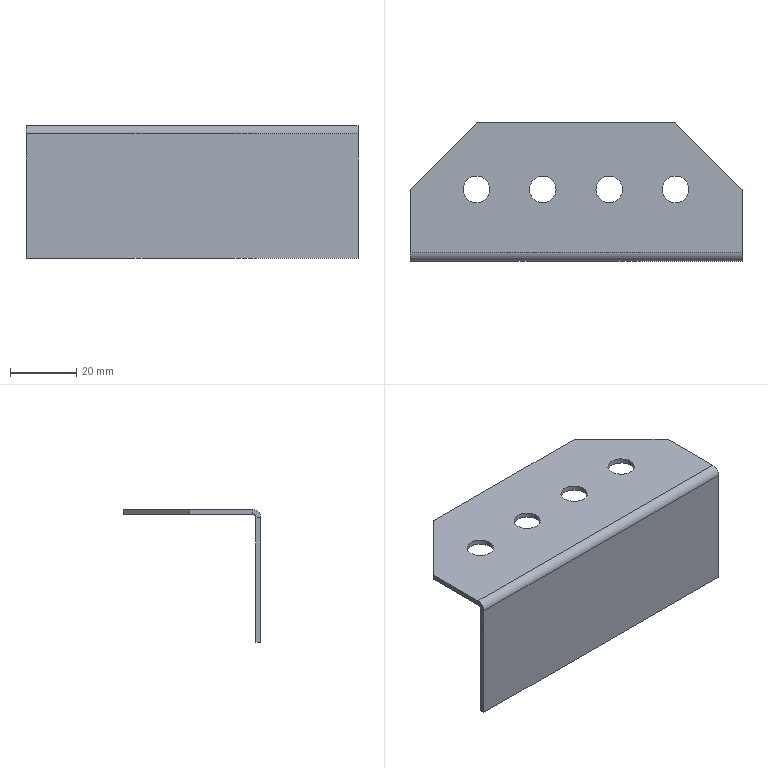Part | SolidWorks | features Chamfer 1, EdgeFlange 1, Extrusion 1, FlatPattern 1, SheetMetal 1, SolidToSheetMetal 1 | 1 solid | 24 faces | box 100 x 41.5 x 40 mm | volume 10986 mm3 | plane 14 | cylinder 10 | commonest cylinder face diameters 8 x8 2 x1 5 x1
STEP:
#1=CARTESIAN_POINT('',(76.,-20.,0.));
#2=VERTEX_POINT('',#1);
#3=CARTESIAN_POINT('',(84.,-20.,0.));
#4=VERTEX_POINT('',#3);
#5=CARTESIAN_POINT('',(80.,-20.,0.));
#6=DIRECTION('',(0.,0.,1.));
#7=DIRECTION('',(1.,0.,0.));
#8=AXIS2_PLACEMENT_3D('',#5,#6,#7);
#9=CIRCLE('',#8,4.);
#10=EDGE_CURVE('',#2,#4,#9,.T.);
#11=ORIENTED_EDGE('',*,*,#10,.F.);
#12=CARTESIAN_POINT('',(76.,-20.,1.5));
#13=VERTEX_POINT('',#12);
#14=CARTESIAN_POINT('',(76.,-20.,1.5));
#15=DIRECTION('',(0.,0.,1.));
#16=VECTOR('',#15,1000.);
#17=LINE('',#14,#16);
#18=EDGE_CURVE('',#2,#13,#17,.T.);
#19=ORIENTED_EDGE('',*,*,#18,.T.);
#20=CARTESIAN_POINT('',(84.,-20.,1.5));
#21=VERTEX_POINT('',#20);
#22=CARTESIAN_POINT('',(80.,-20.,1.5));
#23=DIRECTION('',(0.,0.,1.));
#24=DIRECTION('',(1.,0.,0.));
#25=AXIS2_PLACEMENT_3D('',#22,#23,#24);
#26=CIRCLE('',#25,4.);
#27=EDGE_CURVE('',#13,#21,#26,.T.);
#28=ORIENTED_EDGE('',*,*,#27,.T.);
#29=CARTESIAN_POINT('',(84.,-20.,1.5));
#30=DIRECTION('',(0.,0.,1.));
#31=VECTOR('',#30,1000.);
#32=LINE('',#29,#31);
#33=EDGE_CURVE('',#4,#21,#32,.T.);
#34=ORIENTED_EDGE('',*,*,#33,.F.);
#35=EDGE_LOOP('',(#11,#19,#28,#34));
#36=FACE_OUTER_BOUND('',#35,.T.);
#37=CARTESIAN_POINT('',(80.,-20.,1.5));
#38=DIRECTION('',(0.,0.,1.));
#39=DIRECTION('',(1.,0.,0.));
#40=AXIS2_PLACEMENT_3D('',#37,#38,#39);
#41=CYLINDRICAL_SURFACE('',#40,4.);
#42=ADVANCED_FACE('',(#36),#41,.F.);
#43=CARTESIAN_POINT('',(36.,-20.,0.));
#44=VERTEX_POINT('',#43);
#45=CARTESIAN_POINT('',(44.,-20.,0.));
#46=VERTEX_POINT('',#45);
#47=CARTESIAN_POINT('',(40.,-20.,0.));
#48=DIRECTION('',(0.,0.,1.));
#49=DIRECTION('',(1.,0.,0.));
#50=AXIS2_PLACEMENT_3D('',#47,#48,#49);
#51=CIRCLE('',#50,4.);
#52=EDGE_CURVE('',#44,#46,#51,.T.);
#53=ORIENTED_EDGE('',*,*,#52,.F.);
#54=CARTESIAN_POINT('',(36.,-20.,1.5));
#55=VERTEX_POINT('',#54);
#56=CARTESIAN_POINT('',(36.,-20.,1.5));
#57=DIRECTION('',(0.,0.,1.));
#58=VECTOR('',#57,1000.);
#59=LINE('',#56,#58);
#60=EDGE_CURVE('',#44,#55,#59,.T.);
#61=ORIENTED_EDGE('',*,*,#60,.T.);
#62=CARTESIAN_POINT('',(44.,-20.,1.5));
#63=VERTEX_POINT('',#62);
#64=CARTESIAN_POINT('',(40.,-20.,1.5));
#65=DIRECTION('',(0.,0.,1.));
#66=DIRECTION('',(1.,0.,0.));
#67=AXIS2_PLACEMENT_3D('',#64,#65,#66);
#68=CIRCLE('',#67,4.);
#69=EDGE_CURVE('',#55,#63,#68,.T.);
#70=ORIENTED_EDGE('',*,*,#69,.T.);
#71=CARTESIAN_POINT('',(44.,-20.,1.5));
#72=DIRECTION('',(0.,0.,1.));
#73=VECTOR('',#72,1000.);
#74=LINE('',#71,#73);
#75=EDGE_CURVE('',#46,#63,#74,.T.);
#76=ORIENTED_EDGE('',*,*,#75,.F.);
#77=EDGE_LOOP('',(#53,#61,#70,#76));
#78=FACE_OUTER_BOUND('',#77,.T.);
#79=CARTESIAN_POINT('',(40.,-20.,1.5));
#80=DIRECTION('',(0.,0.,1.));
#81=DIRECTION('',(1.,0.,0.));
#82=AXIS2_PLACEMENT_3D('',#79,#80,#81);
#83=CYLINDRICAL_SURFACE('',#82,4.);
#84=ADVANCED_FACE('',(#78),#83,.F.);
#85=CARTESIAN_POINT('',(16.,-20.,0.));
#86=VERTEX_POINT('',#85);
#87=CARTESIAN_POINT('',(24.,-20.,0.));
#88=VERTEX_POINT('',#87);
#89=CARTESIAN_POINT('',(20.,-20.,0.));
#90=DIRECTION('',(0.,0.,1.));
#91=DIRECTION('',(1.,0.,0.));
#92=AXIS2_PLACEMENT_3D('',#89,#90,#91);
#93=CIRCLE('',#92,4.);
#94=EDGE_CURVE('',#86,#88,#93,.T.);
#95=ORIENTED_EDGE('',*,*,#94,.F.);
#96=CARTESIAN_POINT('',(16.,-20.,1.5));
#97=VERTEX_POINT('',#96);
#98=CARTESIAN_POINT('',(16.,-20.,1.5));
#99=DIRECTION('',(0.,0.,1.));
#100=VECTOR('',#99,1000.);
#101=LINE('',#98,#100);
#102=EDGE_CURVE('',#86,#97,#101,.T.);
#103=ORIENTED_EDGE('',*,*,#102,.T.);
#104=CARTESIAN_POINT('',(24.,-20.,1.5));
#105=VERTEX_POINT('',#104);
#106=CARTESIAN_POINT('',(20.,-20.,1.5));
#107=DIRECTION('',(0.,0.,1.));
#108=DIRECTION('',(1.,0.,0.));
#109=AXIS2_PLACEMENT_3D('',#106,#107,#108);
#110=CIRCLE('',#109,4.);
#111=EDGE_CURVE('',#97,#105,#110,.T.);
#112=ORIENTED_EDGE('',*,*,#111,.T.);
#113=CARTESIAN_POINT('',(24.,-20.,1.5));
#114=DIRECTION('',(0.,0.,1.));
#115=VECTOR('',#114,1000.);
#116=LINE('',#113,#115);
#117=EDGE_CURVE('',#88,#105,#116,.T.);
#118=ORIENTED_EDGE('',*,*,#117,.F.);
#119=EDGE_LOOP('',(#95,#103,#112,#118));
#120=FACE_OUTER_BOUND('',#119,.T.);
#121=CARTESIAN_POINT('',(20.,-20.,1.5));
#122=DIRECTION('',(0.,0.,1.));
#123=DIRECTION('',(1.,0.,0.));
#124=AXIS2_PLACEMENT_3D('',#121,#122,#123);
#125=CYLINDRICAL_SURFACE('',#124,4.);
#126=ADVANCED_FACE('',(#120),#125,.F.);
#127=CARTESIAN_POINT('',(56.,-20.,0.));
#128=VERTEX_POINT('',#127);
#129=CARTESIAN_POINT('',(64.,-20.,0.));
#130=VERTEX_POINT('',#129);
#131=CARTESIAN_POINT('',(60.,-20.,0.));
#132=DIRECTION('',(0.,0.,1.));
#133=DIRECTION('',(1.,0.,0.));
#134=AXIS2_PLACEMENT_3D('',#131,#132,#133);
#135=CIRCLE('',#134,4.);
#136=EDGE_CURVE('',#128,#130,#135,.T.);
#137=ORIENTED_EDGE('',*,*,#136,.F.);
#138=CARTESIAN_POINT('',(56.,-20.,1.5));
#139=VERTEX_POINT('',#138);
#140=CARTESIAN_POINT('',(56.,-20.,1.5));
#141=DIRECTION('',(0.,0.,1.));
#142=VECTOR('',#141,1000.);
#143=LINE('',#140,#142);
#144=EDGE_CURVE('',#128,#139,#143,.T.);
#145=ORIENTED_EDGE('',*,*,#144,.T.);
#146=CARTESIAN_POINT('',(64.,-20.,1.5));
#147=VERTEX_POINT('',#146);
#148=CARTESIAN_POINT('',(60.,-20.,1.5));
#149=DIRECTION('',(0.,0.,1.));
#150=DIRECTION('',(1.,0.,0.));
#151=AXIS2_PLACEMENT_3D('',#148,#149,#150);
#152=CIRCLE('',#151,4.);
#153=EDGE_CURVE('',#139,#147,#152,.T.);
#154=ORIENTED_EDGE('',*,*,#153,.T.);
#155=CARTESIAN_POINT('',(64.,-20.,1.5));
#156=DIRECTION('',(0.,0.,1.));
#157=VECTOR('',#156,1000.);
#158=LINE('',#155,#157);
#159=EDGE_CURVE('',#130,#147,#158,.T.);
#160=ORIENTED_EDGE('',*,*,#159,.F.);
#161=EDGE_LOOP('',(#137,#145,#154,#160));
#162=FACE_OUTER_BOUND('',#161,.T.);
#163=CARTESIAN_POINT('',(60.,-20.,1.5));
#164=DIRECTION('',(0.,0.,1.));
#165=DIRECTION('',(1.,0.,0.));
#166=AXIS2_PLACEMENT_3D('',#163,#164,#165);
#167=CYLINDRICAL_SURFACE('',#166,4.);
#168=ADVANCED_FACE('',(#162),#167,.F.);
#169=CARTESIAN_POINT('',(0.,-20.,0.));
#170=VERTEX_POINT('',#169);
#171=CARTESIAN_POINT('',(0.,-39.,0.));
#172=VERTEX_POINT('',#171);
#173=CARTESIAN_POINT('',(0.,0.,0.));
#174=DIRECTION('',(0.,-1.,0.));
#175=VECTOR('',#174,1000.);
#176=LINE('',#173,#175);
#177=EDGE_CURVE('',#170,#172,#176,.T.);
#178=ORIENTED_EDGE('',*,*,#177,.T.);
#179=CARTESIAN_POINT('',(0.,-39.,1.5));
#180=VERTEX_POINT('',#179);
#181=CARTESIAN_POINT('',(0.,-39.,0.));
#182=DIRECTION('',(0.,0.,1.));
#183=VECTOR('',#182,1000.);
#184=LINE('',#181,#183);
#185=EDGE_CURVE('',#172,#180,#184,.T.);
#186=ORIENTED_EDGE('',*,*,#185,.T.);
#187=CARTESIAN_POINT('',(0.,-20.,1.5));
#188=VERTEX_POINT('',#187);
#189=CARTESIAN_POINT('',(0.,0.,1.5));
#190=DIRECTION('',(0.,-1.,0.));
#191=VECTOR('',#190,1000.);
#192=LINE('',#189,#191);
#193=EDGE_CURVE('',#188,#180,#192,.T.);
#194=ORIENTED_EDGE('',*,*,#193,.F.);
#195=CARTESIAN_POINT('',(0.,-20.,1.5));
#196=DIRECTION('',(0.,0.,1.));
#197=VECTOR('',#196,1000.);
#198=LINE('',#195,#197);
#199=EDGE_CURVE('',#170,#188,#198,.T.);
#200=ORIENTED_EDGE('',*,*,#199,.F.);
#201=EDGE_LOOP('',(#178,#186,#194,#200));
#202=FACE_OUTER_BOUND('',#201,.T.);
#203=CARTESIAN_POINT('',(0.,0.,1.5));
#204=DIRECTION('',(-1.,0.,0.));
#205=DIRECTION('',(0.,-1.,0.));
#206=AXIS2_PLACEMENT_3D('',#203,#204,#205);
#207=PLANE('',#206);
#208=ADVANCED_FACE('',(#202),#207,.T.);
#209=CARTESIAN_POINT('',(60.,-20.,1.5));
#210=DIRECTION('',(0.,0.,1.));
#211=DIRECTION('',(1.,0.,0.));
#212=AXIS2_PLACEMENT_3D('',#209,#210,#211);
#213=CIRCLE('',#212,4.);
#214=EDGE_CURVE('',#147,#139,#213,.T.);
#215=ORIENTED_EDGE('',*,*,#214,.F.);
#216=ORIENTED_EDGE('',*,*,#153,.F.);
#217=EDGE_LOOP('',(#215,#216));
#218=FACE_BOUND('',#217,.T.);
#219=CARTESIAN_POINT('',(20.,-20.,1.5));
#220=DIRECTION('',(0.,0.,1.));
#221=DIRECTION('',(1.,0.,0.));
#222=AXIS2_PLACEMENT_3D('',#219,#220,#221);
#223=CIRCLE('',#222,4.);
#224=EDGE_CURVE('',#105,#97,#223,.T.);
#225=ORIENTED_EDGE('',*,*,#224,.F.);
#226=ORIENTED_EDGE('',*,*,#111,.F.);
#227=EDGE_LOOP('',(#225,#226));
#228=FACE_BOUND('',#227,.T.);
#229=CARTESIAN_POINT('',(40.,-20.,1.5));
#230=DIRECTION('',(0.,0.,1.));
#231=DIRECTION('',(1.,0.,0.));
#232=AXIS2_PLACEMENT_3D('',#229,#230,#231);
#233=CIRCLE('',#232,4.);
#234=EDGE_CURVE('',#63,#55,#233,.T.);
#235=ORIENTED_EDGE('',*,*,#234,.F.);
#236=ORIENTED_EDGE('',*,*,#69,.F.);
#237=EDGE_LOOP('',(#235,#236));
#238=FACE_BOUND('',#237,.T.);
#239=CARTESIAN_POINT('',(80.,-20.,1.5));
#240=DIRECTION('',(0.,0.,1.));
#241=DIRECTION('',(1.,0.,0.));
#242=AXIS2_PLACEMENT_3D('',#239,#240,#241);
#243=CIRCLE('',#242,4.);
#244=EDGE_CURVE('',#21,#13,#243,.T.);
#245=ORIENTED_EDGE('',*,*,#244,.F.);
#246=ORIENTED_EDGE('',*,*,#27,.F.);
#247=EDGE_LOOP('',(#245,#246));
#248=FACE_BOUND('',#247,.T.);
#249=ORIENTED_EDGE('',*,*,#193,.T.);
#250=CARTESIAN_POINT('',(100.,-39.,1.5));
#251=VERTEX_POINT('',#250);
#252=CARTESIAN_POINT('',(0.,-39.,1.5));
#253=DIRECTION('',(1.,0.,0.));
#254=VECTOR('',#253,1000.);
#255=LINE('',#252,#254);
#256=EDGE_CURVE('',#180,#251,#255,.T.);
#257=ORIENTED_EDGE('',*,*,#256,.T.);
#258=CARTESIAN_POINT('',(100.,-20.,1.5));
#259=VERTEX_POINT('',#258);
#260=CARTESIAN_POINT('',(100.,0.,1.5));
#261=DIRECTION('',(0.,1.,0.));
#262=VECTOR('',#261,1000.);
#263=LINE('',#260,#262);
#264=EDGE_CURVE('',#251,#259,#263,.T.);
#265=ORIENTED_EDGE('',*,*,#264,.T.);
#266=CARTESIAN_POINT('',(80.,0.,1.5));
#267=VERTEX_POINT('',#266);
#268=CARTESIAN_POINT('',(40.,40.,1.5));
#269=DIRECTION('',(-0.7071,0.7071,0.));
#270=VECTOR('',#269,1000.);
#271=LINE('',#268,#270);
#272=EDGE_CURVE('',#259,#267,#271,.T.);
#273=ORIENTED_EDGE('',*,*,#272,.T.);
#274=CARTESIAN_POINT('',(20.,0.,1.5));
#275=VERTEX_POINT('',#274);
#276=CARTESIAN_POINT('',(0.,0.,1.5));
#277=DIRECTION('',(-1.,0.,0.));
#278=VECTOR('',#277,1000.);
#279=LINE('',#276,#278);
#280=EDGE_CURVE('',#267,#275,#279,.T.);
#281=ORIENTED_EDGE('',*,*,#280,.T.);
#282=CARTESIAN_POINT('',(10.,-10.,1.5));
#283=DIRECTION('',(-0.7071,-0.7071,0.));
#284=VECTOR('',#283,1000.);
#285=LINE('',#282,#284);
#286=EDGE_CURVE('',#275,#188,#285,.T.);
#287=ORIENTED_EDGE('',*,*,#286,.T.);
#288=EDGE_LOOP('',(#249,#257,#265,#273,#281,#287));
#289=FACE_OUTER_BOUND('',#288,.T.);
#290=CARTESIAN_POINT('',(0.,0.,1.5));
#291=DIRECTION('',(0.,0.,1.));
#292=DIRECTION('',(1.,0.,0.));
#293=AXIS2_PLACEMENT_3D('',#290,#291,#292);
#294=PLANE('',#293);
#295=ADVANCED_FACE('',(#218,#228,#238,#248,#289),#294,.T.);
#296=CARTESIAN_POINT('',(80.,-20.,0.));
#297=DIRECTION('',(0.,0.,1.));
#298=DIRECTION('',(1.,0.,0.));
#299=AXIS2_PLACEMENT_3D('',#296,#297,#298);
#300=CIRCLE('',#299,4.);
#301=EDGE_CURVE('',#4,#2,#300,.T.);
#302=ORIENTED_EDGE('',*,*,#301,.T.);
#303=ORIENTED_EDGE('',*,*,#10,.T.);
#304=EDGE_LOOP('',(#302,#303));
#305=FACE_BOUND('',#304,.T.);
#306=CARTESIAN_POINT('',(40.,-20.,0.));
#307=DIRECTION('',(0.,0.,1.));
#308=DIRECTION('',(1.,0.,0.));
#309=AXIS2_PLACEMENT_3D('',#306,#307,#308);
#310=CIRCLE('',#309,4.);
#311=EDGE_CURVE('',#46,#44,#310,.T.);
#312=ORIENTED_EDGE('',*,*,#311,.T.);
#313=ORIENTED_EDGE('',*,*,#52,.T.);
#314=EDGE_LOOP('',(#312,#313));
#315=FACE_BOUND('',#314,.T.);
#316=CARTESIAN_POINT('',(20.,-20.,0.));
#317=DIRECTION('',(0.,0.,1.));
#318=DIRECTION('',(1.,0.,0.));
#319=AXIS2_PLACEMENT_3D('',#316,#317,#318);
#320=CIRCLE('',#319,4.);
#321=EDGE_CURVE('',#88,#86,#320,.T.);
#322=ORIENTED_EDGE('',*,*,#321,.T.);
#323=ORIENTED_EDGE('',*,*,#94,.T.);
#324=EDGE_LOOP('',(#322,#323));
#325=FACE_BOUND('',#324,.T.);
#326=CARTESIAN_POINT('',(60.,-20.,0.));
#327=DIRECTION('',(0.,0.,1.));
#328=DIRECTION('',(1.,0.,0.));
#329=AXIS2_PLACEMENT_3D('',#326,#327,#328);
#330=CIRCLE('',#329,4.);
#331=EDGE_CURVE('',#130,#128,#330,.T.);
#332=ORIENTED_EDGE('',*,*,#331,.T.);
#333=ORIENTED_EDGE('',*,*,#136,.T.);
#334=EDGE_LOOP('',(#332,#333));
#335=FACE_BOUND('',#334,.T.);
#336=CARTESIAN_POINT('',(100.,-39.,0.));
#337=VERTEX_POINT('',#336);
#338=CARTESIAN_POINT('',(0.,-39.,0.));
#339=DIRECTION('',(1.,0.,0.));
#340=VECTOR('',#339,1000.);
#341=LINE('',#338,#340);
#342=EDGE_CURVE('',#172,#337,#341,.T.);
#343=ORIENTED_EDGE('',*,*,#342,.F.);
#344=ORIENTED_EDGE('',*,*,#177,.F.);
#345=CARTESIAN_POINT('',(20.,0.,0.));
#346=VERTEX_POINT('',#345);
#347=CARTESIAN_POINT('',(10.,-10.,0.));
#348=DIRECTION('',(-0.7071,-0.7071,0.));
#349=VECTOR('',#348,1000.);
#350=LINE('',#347,#349);
#351=EDGE_CURVE('',#346,#170,#350,.T.);
#352=ORIENTED_EDGE('',*,*,#351,.F.);
#353=CARTESIAN_POINT('',(80.,0.,0.));
#354=VERTEX_POINT('',#353);
#355=CARTESIAN_POINT('',(0.,0.,0.));
#356=DIRECTION('',(-1.,0.,0.));
#357=VECTOR('',#356,1000.);
#358=LINE('',#355,#357);
#359=EDGE_CURVE('',#354,#346,#358,.T.);
#360=ORIENTED_EDGE('',*,*,#359,.F.);
#361=CARTESIAN_POINT('',(100.,-20.,0.));
#362=VERTEX_POINT('',#361);
#363=CARTESIAN_POINT('',(40.,40.,0.));
#364=DIRECTION('',(-0.7071,0.7071,0.));
#365=VECTOR('',#364,1000.);
#366=LINE('',#363,#365);
#367=EDGE_CURVE('',#362,#354,#366,.T.);
#368=ORIENTED_EDGE('',*,*,#367,.F.);
#369=CARTESIAN_POINT('',(100.,0.,0.));
#370=DIRECTION('',(0.,1.,0.));
#371=VECTOR('',#370,1000.);
#372=LINE('',#369,#371);
#373=EDGE_CURVE('',#337,#362,#372,.T.);
#374=ORIENTED_EDGE('',*,*,#373,.F.);
#375=EDGE_LOOP('',(#343,#344,#352,#360,#368,#374));
#376=FACE_OUTER_BOUND('',#375,.T.);
#377=CARTESIAN_POINT('',(0.,0.,0.));
#378=DIRECTION('',(0.,0.,1.));
#379=DIRECTION('',(1.,0.,0.));
#380=AXIS2_PLACEMENT_3D('',#377,#378,#379);
#381=PLANE('',#380);
#382=ADVANCED_FACE('',(#305,#315,#325,#335,#376),#381,.F.);
#383=CARTESIAN_POINT('',(80.,0.,1.5));
#384=DIRECTION('',(0.,0.,1.));
#385=VECTOR('',#384,1000.);
#386=LINE('',#383,#385);
#387=EDGE_CURVE('',#354,#267,#386,.T.);
#388=ORIENTED_EDGE('',*,*,#387,.F.);
#389=ORIENTED_EDGE('',*,*,#359,.T.);
#390=CARTESIAN_POINT('',(20.,0.,1.5));
#391=DIRECTION('',(0.,0.,1.));
#392=VECTOR('',#391,1000.);
#393=LINE('',#390,#392);
#394=EDGE_CURVE('',#346,#275,#393,.T.);
#395=ORIENTED_EDGE('',*,*,#394,.T.);
#396=ORIENTED_EDGE('',*,*,#280,.F.);
#397=EDGE_LOOP('',(#388,#389,#395,#396));
#398=FACE_OUTER_BOUND('',#397,.T.);
#399=CARTESIAN_POINT('',(0.,0.,1.5));
#400=DIRECTION('',(0.,1.,0.));
#401=DIRECTION('',(-1.,0.,0.));
#402=AXIS2_PLACEMENT_3D('',#399,#400,#401);
#403=PLANE('',#402);
#404=ADVANCED_FACE('',(#398),#403,.T.);
#405=ORIENTED_EDGE('',*,*,#394,.F.);
#406=ORIENTED_EDGE('',*,*,#351,.T.);
#407=ORIENTED_EDGE('',*,*,#199,.T.);
#408=ORIENTED_EDGE('',*,*,#286,.F.);
#409=EDGE_LOOP('',(#405,#406,#407,#408));
#410=FACE_OUTER_BOUND('',#409,.T.);
#411=CARTESIAN_POINT('',(10.,-10.,1.5));
#412=DIRECTION('',(0.7071,-0.7071,0.));
#413=DIRECTION('',(0.7071,0.7071,0.));
#414=AXIS2_PLACEMENT_3D('',#411,#412,#413);
#415=PLANE('',#414);
#416=ADVANCED_FACE('',(#410),#415,.F.);
#417=CARTESIAN_POINT('',(100.,-39.,0.));
#418=DIRECTION('',(0.,0.,1.));
#419=VECTOR('',#418,1000.);
#420=LINE('',#417,#419);
#421=EDGE_CURVE('',#337,#251,#420,.T.);
#422=ORIENTED_EDGE('',*,*,#421,.F.);
#423=ORIENTED_EDGE('',*,*,#373,.T.);
#424=CARTESIAN_POINT('',(100.,-20.,1.5));
#425=DIRECTION('',(0.,0.,1.));
#426=VECTOR('',#425,1000.);
#427=LINE('',#424,#426);
#428=EDGE_CURVE('',#362,#259,#427,.T.);
#429=ORIENTED_EDGE('',*,*,#428,.T.);
#430=ORIENTED_EDGE('',*,*,#264,.F.);
#431=EDGE_LOOP('',(#422,#423,#429,#430));
#432=FACE_OUTER_BOUND('',#431,.T.);
#433=CARTESIAN_POINT('',(100.,0.,1.5));
#434=DIRECTION('',(1.,0.,0.));
#435=DIRECTION('',(0.,1.,0.));
#436=AXIS2_PLACEMENT_3D('',#433,#434,#435);
#437=PLANE('',#436);
#438=ADVANCED_FACE('',(#432),#437,.T.);
#439=ORIENTED_EDGE('',*,*,#144,.F.);
#440=ORIENTED_EDGE('',*,*,#331,.F.);
#441=ORIENTED_EDGE('',*,*,#159,.T.);
#442=ORIENTED_EDGE('',*,*,#214,.T.);
#443=EDGE_LOOP('',(#439,#440,#441,#442));
#444=FACE_OUTER_BOUND('',#443,.T.);
#445=CARTESIAN_POINT('',(60.,-20.,1.5));
#446=DIRECTION('',(0.,0.,1.));
#447=DIRECTION('',(1.,0.,0.));
#448=AXIS2_PLACEMENT_3D('',#445,#446,#447);
#449=CYLINDRICAL_SURFACE('',#448,4.);
#450=ADVANCED_FACE('',(#444),#449,.F.);
#451=ORIENTED_EDGE('',*,*,#102,.F.);
#452=ORIENTED_EDGE('',*,*,#321,.F.);
#453=ORIENTED_EDGE('',*,*,#117,.T.);
#454=ORIENTED_EDGE('',*,*,#224,.T.);
#455=EDGE_LOOP('',(#451,#452,#453,#454));
#456=FACE_OUTER_BOUND('',#455,.T.);
#457=CARTESIAN_POINT('',(20.,-20.,1.5));
#458=DIRECTION('',(0.,0.,1.));
#459=DIRECTION('',(1.,0.,0.));
#460=AXIS2_PLACEMENT_3D('',#457,#458,#459);
#461=CYLINDRICAL_SURFACE('',#460,4.);
#462=ADVANCED_FACE('',(#456),#461,.F.);
#463=ORIENTED_EDGE('',*,*,#367,.T.);
#464=ORIENTED_EDGE('',*,*,#387,.T.);
#465=ORIENTED_EDGE('',*,*,#272,.F.);
#466=ORIENTED_EDGE('',*,*,#428,.F.);
#467=EDGE_LOOP('',(#463,#464,#465,#466));
#468=FACE_OUTER_BOUND('',#467,.T.);
#469=CARTESIAN_POINT('',(40.,40.,1.5));
#470=DIRECTION('',(-0.7071,-0.7071,0.));
#471=DIRECTION('',(0.7071,-0.7071,0.));
#472=AXIS2_PLACEMENT_3D('',#469,#470,#471);
#473=PLANE('',#472);
#474=ADVANCED_FACE('',(#468),#473,.F.);
#475=ORIENTED_EDGE('',*,*,#60,.F.);
#476=ORIENTED_EDGE('',*,*,#311,.F.);
#477=ORIENTED_EDGE('',*,*,#75,.T.);
#478=ORIENTED_EDGE('',*,*,#234,.T.);
#479=EDGE_LOOP('',(#475,#476,#477,#478));
#480=FACE_OUTER_BOUND('',#479,.T.);
#481=CARTESIAN_POINT('',(40.,-20.,1.5));
#482=DIRECTION('',(0.,0.,1.));
#483=DIRECTION('',(1.,0.,0.));
#484=AXIS2_PLACEMENT_3D('',#481,#482,#483);
#485=CYLINDRICAL_SURFACE('',#484,4.);
#486=ADVANCED_FACE('',(#480),#485,.F.);
#487=ORIENTED_EDGE('',*,*,#18,.F.);
#488=ORIENTED_EDGE('',*,*,#301,.F.);
#489=ORIENTED_EDGE('',*,*,#33,.T.);
#490=ORIENTED_EDGE('',*,*,#244,.T.);
#491=EDGE_LOOP('',(#487,#488,#489,#490));
#492=FACE_OUTER_BOUND('',#491,.T.);
#493=CARTESIAN_POINT('',(80.,-20.,1.5));
#494=DIRECTION('',(0.,0.,1.));
#495=DIRECTION('',(1.,0.,0.));
#496=AXIS2_PLACEMENT_3D('',#493,#494,#495);
#497=CYLINDRICAL_SURFACE('',#496,4.);
#498=ADVANCED_FACE('',(#492),#497,.F.);
#499=CARTESIAN_POINT('',(100.,-40.,-1.));
#500=VERTEX_POINT('',#499);
#501=CARTESIAN_POINT('',(100.,-41.5,-1.));
#502=VERTEX_POINT('',#501);
#503=CARTESIAN_POINT('',(100.,-40.,-1.));
#504=DIRECTION('',(0.,-1.,0.));
#505=VECTOR('',#504,1000.);
#506=LINE('',#503,#505);
#507=EDGE_CURVE('',#500,#502,#506,.T.);
#508=ORIENTED_EDGE('',*,*,#507,.F.);
#509=CARTESIAN_POINT('',(100.,-39.,-1.));
#510=DIRECTION('',(1.,0.,0.));
#511=DIRECTION('',(0.,0.,1.));
#512=AXIS2_PLACEMENT_3D('',#509,#510,#511);
#513=CIRCLE('',#512,1.);
#514=EDGE_CURVE('',#337,#500,#513,.T.);
#515=ORIENTED_EDGE('',*,*,#514,.F.);
#516=ORIENTED_EDGE('',*,*,#421,.T.);
#517=CARTESIAN_POINT('',(100.,-39.,-1.));
#518=DIRECTION('',(1.,0.,0.));
#519=DIRECTION('',(0.,0.,1.));
#520=AXIS2_PLACEMENT_3D('',#517,#518,#519);
#521=CIRCLE('',#520,2.5);
#522=EDGE_CURVE('',#251,#502,#521,.T.);
#523=ORIENTED_EDGE('',*,*,#522,.T.);
#524=EDGE_LOOP('',(#508,#515,#516,#523));
#525=FACE_OUTER_BOUND('',#524,.T.);
#526=CARTESIAN_POINT('',(100.,-39.,-1.));
#527=DIRECTION('',(1.,0.,0.));
#528=DIRECTION('',(0.,0.,-1.));
#529=AXIS2_PLACEMENT_3D('',#526,#527,#528);
#530=PLANE('',#529);
#531=ADVANCED_FACE('',(#525),#530,.T.);
#532=CARTESIAN_POINT('',(0.,-40.,-1.));
#533=VERTEX_POINT('',#532);
#534=CARTESIAN_POINT('',(0.,-39.,-1.));
#535=DIRECTION('',(-1.,0.,0.));
#536=DIRECTION('',(0.,0.,1.));
#537=AXIS2_PLACEMENT_3D('',#534,#535,#536);
#538=CIRCLE('',#537,1.);
#539=EDGE_CURVE('',#533,#172,#538,.T.);
#540=ORIENTED_EDGE('',*,*,#539,.F.);
#541=CARTESIAN_POINT('',(0.,-41.5,-1.));
#542=VERTEX_POINT('',#541);
#543=CARTESIAN_POINT('',(0.,-40.,-1.));
#544=DIRECTION('',(0.,-1.,0.));
#545=VECTOR('',#544,1000.);
#546=LINE('',#543,#545);
#547=EDGE_CURVE('',#533,#542,#546,.T.);
#548=ORIENTED_EDGE('',*,*,#547,.T.);
#549=CARTESIAN_POINT('',(0.,-39.,-1.));
#550=DIRECTION('',(-1.,0.,0.));
#551=DIRECTION('',(0.,0.,1.));
#552=AXIS2_PLACEMENT_3D('',#549,#550,#551);
#553=CIRCLE('',#552,2.5);
#554=EDGE_CURVE('',#542,#180,#553,.T.);
#555=ORIENTED_EDGE('',*,*,#554,.T.);
#556=ORIENTED_EDGE('',*,*,#185,.F.);
#557=EDGE_LOOP('',(#540,#548,#555,#556));
#558=FACE_OUTER_BOUND('',#557,.T.);
#559=CARTESIAN_POINT('',(0.,-39.,-1.));
#560=DIRECTION('',(1.,0.,0.));
#561=DIRECTION('',(0.,0.,-1.));
#562=AXIS2_PLACEMENT_3D('',#559,#560,#561);
#563=PLANE('',#562);
#564=ADVANCED_FACE('',(#558),#563,.F.);
#565=ORIENTED_EDGE('',*,*,#256,.F.);
#566=ORIENTED_EDGE('',*,*,#554,.F.);
#567=CARTESIAN_POINT('',(0.,-41.5,-1.));
#568=DIRECTION('',(-1.,0.,0.));
#569=VECTOR('',#568,1000.);
#570=LINE('',#567,#569);
#571=EDGE_CURVE('',#502,#542,#570,.T.);
#572=ORIENTED_EDGE('',*,*,#571,.F.);
#573=ORIENTED_EDGE('',*,*,#522,.F.);
#574=EDGE_LOOP('',(#565,#566,#572,#573));
#575=FACE_OUTER_BOUND('',#574,.T.);
#576=CARTESIAN_POINT('',(0.,-39.,-1.));
#577=DIRECTION('',(-1.,0.,0.));
#578=DIRECTION('',(0.,-1.,0.));
#579=AXIS2_PLACEMENT_3D('',#576,#577,#578);
#580=CYLINDRICAL_SURFACE('',#579,2.5);
#581=ADVANCED_FACE('',(#575),#580,.T.);
#582=ORIENTED_EDGE('',*,*,#342,.T.);
#583=ORIENTED_EDGE('',*,*,#514,.T.);
#584=CARTESIAN_POINT('',(100.,-40.,-1.));
#585=DIRECTION('',(-1.,0.,0.));
#586=VECTOR('',#585,1000.);
#587=LINE('',#584,#586);
#588=EDGE_CURVE('',#500,#533,#587,.T.);
#589=ORIENTED_EDGE('',*,*,#588,.T.);
#590=ORIENTED_EDGE('',*,*,#539,.T.);
#591=EDGE_LOOP('',(#582,#583,#589,#590));
#592=FACE_OUTER_BOUND('',#591,.T.);
#593=CARTESIAN_POINT('',(0.,-39.,-1.));
#594=DIRECTION('',(-1.,0.,0.));
#595=DIRECTION('',(0.,-1.,0.));
#596=AXIS2_PLACEMENT_3D('',#593,#594,#595);
#597=CYLINDRICAL_SURFACE('',#596,1.);
#598=ADVANCED_FACE('',(#592),#597,.F.);
#599=CARTESIAN_POINT('',(0.,-41.5,-38.5));
#600=VERTEX_POINT('',#599);
#601=CARTESIAN_POINT('',(0.,-41.5,0.));
#602=DIRECTION('',(0.,0.,1.));
#603=VECTOR('',#602,1000.);
#604=LINE('',#601,#603);
#605=EDGE_CURVE('',#600,#542,#604,.T.);
#606=ORIENTED_EDGE('',*,*,#605,.T.);
#607=ORIENTED_EDGE('',*,*,#547,.F.);
#608=CARTESIAN_POINT('',(0.,-40.,-38.5));
#609=VERTEX_POINT('',#608);
#610=CARTESIAN_POINT('',(0.,-40.,0.));
#611=DIRECTION('',(0.,0.,1.));
#612=VECTOR('',#611,1000.);
#613=LINE('',#610,#612);
#614=EDGE_CURVE('',#609,#533,#613,.T.);
#615=ORIENTED_EDGE('',*,*,#614,.F.);
#616=CARTESIAN_POINT('',(0.,-41.5,-38.5));
#617=DIRECTION('',(0.,1.,0.));
#618=VECTOR('',#617,1000.);
#619=LINE('',#616,#618);
#620=EDGE_CURVE('',#600,#609,#619,.T.);
#621=ORIENTED_EDGE('',*,*,#620,.F.);
#622=EDGE_LOOP('',(#606,#607,#615,#621));
#623=FACE_OUTER_BOUND('',#622,.T.);
#624=CARTESIAN_POINT('',(0.,-41.5,0.));
#625=DIRECTION('',(-1.,0.,0.));
#626=DIRECTION('',(0.,0.,1.));
#627=AXIS2_PLACEMENT_3D('',#624,#625,#626);
#628=PLANE('',#627);
#629=ADVANCED_FACE('',(#623),#628,.T.);
#630=CARTESIAN_POINT('',(100.,-40.,-38.5));
#631=VERTEX_POINT('',#630);
#632=CARTESIAN_POINT('',(100.,-40.,-38.5));
#633=DIRECTION('',(0.,0.,-1.));
#634=VECTOR('',#633,1000.);
#635=LINE('',#632,#634);
#636=EDGE_CURVE('',#500,#631,#635,.T.);
#637=ORIENTED_EDGE('',*,*,#636,.F.);
#638=ORIENTED_EDGE('',*,*,#507,.T.);
#639=CARTESIAN_POINT('',(100.,-41.5,-38.5));
#640=VERTEX_POINT('',#639);
#641=CARTESIAN_POINT('',(100.,-41.5,-38.5));
#642=DIRECTION('',(0.,0.,-1.));
#643=VECTOR('',#642,1000.);
#644=LINE('',#641,#643);
#645=EDGE_CURVE('',#502,#640,#644,.T.);
#646=ORIENTED_EDGE('',*,*,#645,.T.);
#647=CARTESIAN_POINT('',(100.,-41.5,-38.5));
#648=DIRECTION('',(0.,1.,0.));
#649=VECTOR('',#648,1000.);
#650=LINE('',#647,#649);
#651=EDGE_CURVE('',#640,#631,#650,.T.);
#652=ORIENTED_EDGE('',*,*,#651,.T.);
#653=EDGE_LOOP('',(#637,#638,#646,#652));
#654=FACE_OUTER_BOUND('',#653,.T.);
#655=CARTESIAN_POINT('',(100.,-41.5,-38.5));
#656=DIRECTION('',(1.,0.,0.));
#657=DIRECTION('',(0.,0.,-1.));
#658=AXIS2_PLACEMENT_3D('',#655,#656,#657);
#659=PLANE('',#658);
#660=ADVANCED_FACE('',(#654),#659,.T.);
#661=ORIENTED_EDGE('',*,*,#645,.F.);
#662=ORIENTED_EDGE('',*,*,#571,.T.);
#663=ORIENTED_EDGE('',*,*,#605,.F.);
#664=CARTESIAN_POINT('',(0.,-41.5,-38.5));
#665=DIRECTION('',(-1.,0.,0.));
#666=VECTOR('',#665,1000.);
#667=LINE('',#664,#666);
#668=EDGE_CURVE('',#640,#600,#667,.T.);
#669=ORIENTED_EDGE('',*,*,#668,.F.);
#670=EDGE_LOOP('',(#661,#662,#663,#669));
#671=FACE_OUTER_BOUND('',#670,.T.);
#672=CARTESIAN_POINT('',(0.,-41.5,0.));
#673=DIRECTION('',(0.,-1.,0.));
#674=DIRECTION('',(0.,0.,-1.));
#675=AXIS2_PLACEMENT_3D('',#672,#673,#674);
#676=PLANE('',#675);
#677=ADVANCED_FACE('',(#671),#676,.T.);
#678=ORIENTED_EDGE('',*,*,#588,.F.);
#679=ORIENTED_EDGE('',*,*,#636,.T.);
#680=CARTESIAN_POINT('',(0.,-40.,-38.5));
#681=DIRECTION('',(-1.,0.,0.));
#682=VECTOR('',#681,1000.);
#683=LINE('',#680,#682);
#684=EDGE_CURVE('',#631,#609,#683,.T.);
#685=ORIENTED_EDGE('',*,*,#684,.T.);
#686=ORIENTED_EDGE('',*,*,#614,.T.);
#687=EDGE_LOOP('',(#678,#679,#685,#686));
#688=FACE_OUTER_BOUND('',#687,.T.);
#689=CARTESIAN_POINT('',(0.,-40.,0.));
#690=DIRECTION('',(0.,-1.,0.));
#691=DIRECTION('',(0.,0.,-1.));
#692=AXIS2_PLACEMENT_3D('',#689,#690,#691);
#693=PLANE('',#692);
#694=ADVANCED_FACE('',(#688),#693,.F.);
#695=ORIENTED_EDGE('',*,*,#684,.F.);
#696=ORIENTED_EDGE('',*,*,#651,.F.);
#697=ORIENTED_EDGE('',*,*,#668,.T.);
#698=ORIENTED_EDGE('',*,*,#620,.T.);
#699=EDGE_LOOP('',(#695,#696,#697,#698));
#700=FACE_OUTER_BOUND('',#699,.T.);
#701=CARTESIAN_POINT('',(0.,-41.5,-38.5));
#702=DIRECTION('',(0.,0.,-1.));
#703=DIRECTION('',(0.,1.,0.));
#704=AXIS2_PLACEMENT_3D('',#701,#702,#703);
#705=PLANE('',#704);
#706=ADVANCED_FACE('',(#700),#705,.T.);
#707=CLOSED_SHELL('',(#42,#84,#126,#168,#208,#295,#382,#404,#416,#438,#450,#462,#474,#486,#498,#531,#564,#581,#598,#629,#660,#677,#694,#706));
#708=MANIFOLD_SOLID_BREP('',#707);
#709=CARTESIAN_POINT('',(0.,0.,0.));
#710=DIRECTION('',(0.,0.,1.));
#711=DIRECTION('',(1.,0.,0.));
#712=AXIS2_PLACEMENT_3D('',#709,#710,#711);
#713=(LENGTH_UNIT()NAMED_UNIT(*)SI_UNIT(.MILLI.,.METRE.));
#714=UNCERTAINTY_MEASURE_WITH_UNIT(LENGTH_MEASURE(0.00001),#713,'','');
#715=(NAMED_UNIT(*)PLANE_ANGLE_UNIT()SI_UNIT($,.RADIAN.));
#716=(NAMED_UNIT(*)SI_UNIT($,.STERADIAN.)SOLID_ANGLE_UNIT());
#717=(GEOMETRIC_REPRESENTATION_CONTEXT(3)GLOBAL_UNCERTAINTY_ASSIGNED_CONTEXT((#714))GLOBAL_UNIT_ASSIGNED_CONTEXT((#713,#715,#716))REPRESENTATION_CONTEXT('',''));
#718=ADVANCED_BREP_SHAPE_REPRESENTATION('',(#708,#712),#717);